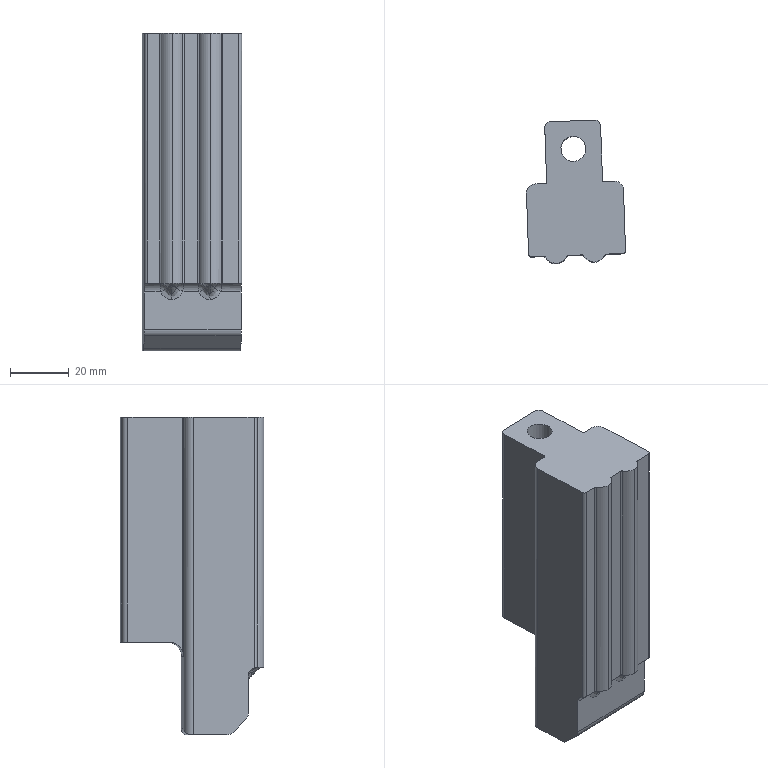Part | NX | features PU-11 2 | 1 solid | 56 faces | box 33.703 x 48.735 x 108 mm | volume 111549 mm3 | cylinder 21 | spline 16 | plane 15 | sphere 4 | commonest cylinder face diameters 6 x7 1 x6 4 x3 2 x2 8.506 x1 10 x1